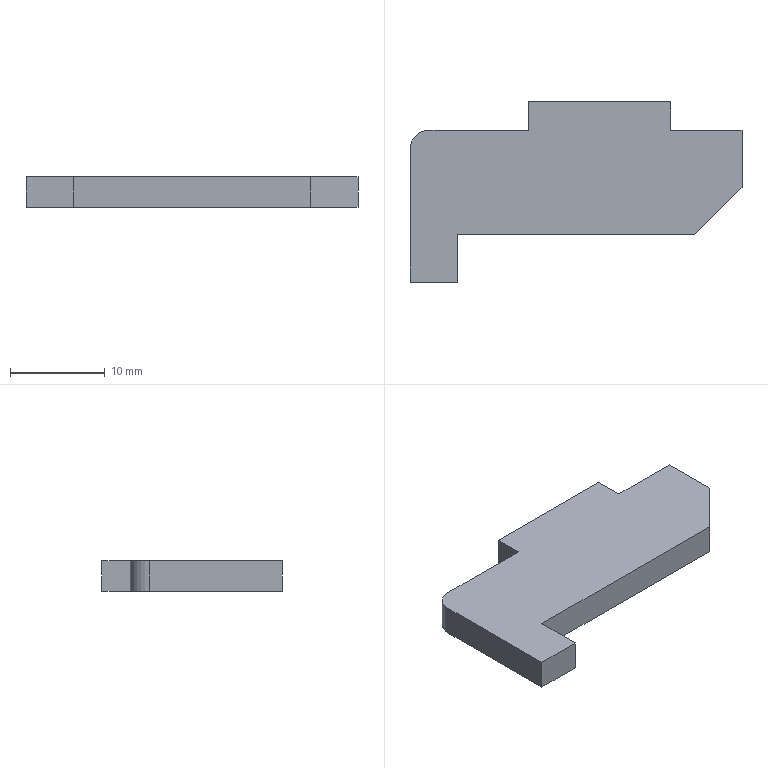Part | SolidWorks | features FlatPattern 1, SMBaseFlange 1, SheetMetal 1 | 1 solid | 14 faces | box 35 x 19 x 3.2 mm | volume 1413 mm3 | plane 13 | cylinder 1 | commonest cylinder face diameters 4 x1
STEP:
#1=CARTESIAN_POINT('',(-81.748,-105.118,0.));
#2=VERTEX_POINT('',#1);
#3=CARTESIAN_POINT('',(-81.748,-100.118,0.));
#4=VERTEX_POINT('',#3);
#5=CARTESIAN_POINT('',(-81.748,-100.118,0.));
#6=DIRECTION('',(0.,1.,0.));
#7=VECTOR('',#6,1000.);
#8=LINE('',#5,#7);
#9=EDGE_CURVE('',#2,#4,#8,.T.);
#10=ORIENTED_EDGE('',*,*,#9,.F.);
#11=CARTESIAN_POINT('',(-81.748,-105.118,-3.2));
#12=VERTEX_POINT('',#11);
#13=CARTESIAN_POINT('',(-81.748,-105.118,-3.2));
#14=DIRECTION('',(0.,0.,1.));
#15=VECTOR('',#14,1000.);
#16=LINE('',#13,#15);
#17=EDGE_CURVE('',#12,#2,#16,.T.);
#18=ORIENTED_EDGE('',*,*,#17,.F.);
#19=CARTESIAN_POINT('',(-81.748,-100.118,-3.2));
#20=VERTEX_POINT('',#19);
#21=CARTESIAN_POINT('',(-81.748,-100.118,-3.2));
#22=DIRECTION('',(0.,1.,0.));
#23=VECTOR('',#22,1000.);
#24=LINE('',#21,#23);
#25=EDGE_CURVE('',#12,#20,#24,.T.);
#26=ORIENTED_EDGE('',*,*,#25,.T.);
#27=CARTESIAN_POINT('',(-81.748,-100.118,-3.2));
#28=DIRECTION('',(0.,0.,1.));
#29=VECTOR('',#28,1000.);
#30=LINE('',#27,#29);
#31=EDGE_CURVE('',#20,#4,#30,.T.);
#32=ORIENTED_EDGE('',*,*,#31,.T.);
#33=EDGE_LOOP('',(#10,#18,#26,#32));
#34=FACE_OUTER_BOUND('',#33,.T.);
#35=CARTESIAN_POINT('',(-81.748,-100.118,-3.2));
#36=DIRECTION('',(1.,0.,0.));
#37=DIRECTION('',(0.,0.,-1.));
#38=AXIS2_PLACEMENT_3D('',#35,#36,#37);
#39=PLANE('',#38);
#40=ADVANCED_FACE('',(#34),#39,.T.);
#41=CARTESIAN_POINT('',(-86.748,-105.118,0.));
#42=VERTEX_POINT('',#41);
#43=CARTESIAN_POINT('',(-81.748,-105.118,0.));
#44=DIRECTION('',(1.,0.,0.));
#45=VECTOR('',#44,1000.);
#46=LINE('',#43,#45);
#47=EDGE_CURVE('',#42,#2,#46,.T.);
#48=ORIENTED_EDGE('',*,*,#47,.F.);
#49=CARTESIAN_POINT('',(-86.748,-105.118,-3.2));
#50=VERTEX_POINT('',#49);
#51=CARTESIAN_POINT('',(-86.748,-105.118,-3.2));
#52=DIRECTION('',(0.,0.,1.));
#53=VECTOR('',#52,1000.);
#54=LINE('',#51,#53);
#55=EDGE_CURVE('',#50,#42,#54,.T.);
#56=ORIENTED_EDGE('',*,*,#55,.F.);
#57=CARTESIAN_POINT('',(-81.748,-105.118,-3.2));
#58=DIRECTION('',(1.,0.,0.));
#59=VECTOR('',#58,1000.);
#60=LINE('',#57,#59);
#61=EDGE_CURVE('',#50,#12,#60,.T.);
#62=ORIENTED_EDGE('',*,*,#61,.T.);
#63=ORIENTED_EDGE('',*,*,#17,.T.);
#64=EDGE_LOOP('',(#48,#56,#62,#63));
#65=FACE_OUTER_BOUND('',#64,.T.);
#66=CARTESIAN_POINT('',(-81.748,-105.118,-3.2));
#67=DIRECTION('',(0.,-1.,0.));
#68=DIRECTION('',(0.,0.,-1.));
#69=AXIS2_PLACEMENT_3D('',#66,#67,#68);
#70=PLANE('',#69);
#71=ADVANCED_FACE('',(#65),#70,.T.);
#72=CARTESIAN_POINT('',(-86.748,-91.118,0.));
#73=VERTEX_POINT('',#72);
#74=CARTESIAN_POINT('',(-86.748,-105.118,0.));
#75=DIRECTION('',(0.,-1.,0.));
#76=VECTOR('',#75,1000.);
#77=LINE('',#74,#76);
#78=EDGE_CURVE('',#73,#42,#77,.T.);
#79=ORIENTED_EDGE('',*,*,#78,.F.);
#80=CARTESIAN_POINT('',(-86.748,-91.118,-3.2));
#81=VERTEX_POINT('',#80);
#82=CARTESIAN_POINT('',(-86.748,-91.118,-3.2));
#83=DIRECTION('',(0.,0.,1.));
#84=VECTOR('',#83,1000.);
#85=LINE('',#82,#84);
#86=EDGE_CURVE('',#81,#73,#85,.T.);
#87=ORIENTED_EDGE('',*,*,#86,.F.);
#88=CARTESIAN_POINT('',(-86.748,-105.118,-3.2));
#89=DIRECTION('',(0.,-1.,0.));
#90=VECTOR('',#89,1000.);
#91=LINE('',#88,#90);
#92=EDGE_CURVE('',#81,#50,#91,.T.);
#93=ORIENTED_EDGE('',*,*,#92,.T.);
#94=ORIENTED_EDGE('',*,*,#55,.T.);
#95=EDGE_LOOP('',(#79,#87,#93,#94));
#96=FACE_OUTER_BOUND('',#95,.T.);
#97=CARTESIAN_POINT('',(-86.748,-105.118,-3.2));
#98=DIRECTION('',(-1.,0.,0.));
#99=DIRECTION('',(0.,0.,1.));
#100=AXIS2_PLACEMENT_3D('',#97,#98,#99);
#101=PLANE('',#100);
#102=ADVANCED_FACE('',(#96),#101,.T.);
#103=CARTESIAN_POINT('',(-84.748,-89.118,0.));
#104=VERTEX_POINT('',#103);
#105=CARTESIAN_POINT('',(-84.748,-91.118,0.));
#106=DIRECTION('',(0.,0.,1.));
#107=DIRECTION('',(-1.,0.,0.));
#108=AXIS2_PLACEMENT_3D('',#105,#106,#107);
#109=CIRCLE('',#108,2.);
#110=EDGE_CURVE('',#104,#73,#109,.T.);
#111=ORIENTED_EDGE('',*,*,#110,.F.);
#112=CARTESIAN_POINT('',(-84.748,-89.118,-3.2));
#113=VERTEX_POINT('',#112);
#114=CARTESIAN_POINT('',(-84.748,-89.118,-3.2));
#115=DIRECTION('',(0.,0.,1.));
#116=VECTOR('',#115,1000.);
#117=LINE('',#114,#116);
#118=EDGE_CURVE('',#113,#104,#117,.T.);
#119=ORIENTED_EDGE('',*,*,#118,.F.);
#120=CARTESIAN_POINT('',(-84.748,-91.118,-3.2));
#121=DIRECTION('',(0.,0.,1.));
#122=DIRECTION('',(-1.,0.,0.));
#123=AXIS2_PLACEMENT_3D('',#120,#121,#122);
#124=CIRCLE('',#123,2.);
#125=EDGE_CURVE('',#113,#81,#124,.T.);
#126=ORIENTED_EDGE('',*,*,#125,.T.);
#127=ORIENTED_EDGE('',*,*,#86,.T.);
#128=EDGE_LOOP('',(#111,#119,#126,#127));
#129=FACE_OUTER_BOUND('',#128,.T.);
#130=CARTESIAN_POINT('',(-84.748,-91.118,-3.2));
#131=DIRECTION('',(0.,0.,1.));
#132=DIRECTION('',(1.,0.,0.));
#133=AXIS2_PLACEMENT_3D('',#130,#131,#132);
#134=CYLINDRICAL_SURFACE('',#133,2.);
#135=ADVANCED_FACE('',(#129),#134,.T.);
#136=CARTESIAN_POINT('',(-74.248,-89.118,0.));
#137=VERTEX_POINT('',#136);
#138=CARTESIAN_POINT('',(-84.748,-89.118,0.));
#139=DIRECTION('',(-1.,0.,0.));
#140=VECTOR('',#139,1000.);
#141=LINE('',#138,#140);
#142=EDGE_CURVE('',#137,#104,#141,.T.);
#143=ORIENTED_EDGE('',*,*,#142,.F.);
#144=CARTESIAN_POINT('',(-74.248,-89.118,-3.2));
#145=VERTEX_POINT('',#144);
#146=CARTESIAN_POINT('',(-74.248,-89.118,-3.2));
#147=DIRECTION('',(0.,0.,1.));
#148=VECTOR('',#147,1000.);
#149=LINE('',#146,#148);
#150=EDGE_CURVE('',#145,#137,#149,.T.);
#151=ORIENTED_EDGE('',*,*,#150,.F.);
#152=CARTESIAN_POINT('',(-84.748,-89.118,-3.2));
#153=DIRECTION('',(-1.,0.,0.));
#154=VECTOR('',#153,1000.);
#155=LINE('',#152,#154);
#156=EDGE_CURVE('',#145,#113,#155,.T.);
#157=ORIENTED_EDGE('',*,*,#156,.T.);
#158=ORIENTED_EDGE('',*,*,#118,.T.);
#159=EDGE_LOOP('',(#143,#151,#157,#158));
#160=FACE_OUTER_BOUND('',#159,.T.);
#161=CARTESIAN_POINT('',(-84.748,-89.118,-3.2));
#162=DIRECTION('',(0.,1.,0.));
#163=DIRECTION('',(0.,0.,1.));
#164=AXIS2_PLACEMENT_3D('',#161,#162,#163);
#165=PLANE('',#164);
#166=ADVANCED_FACE('',(#160),#165,.T.);
#167=CARTESIAN_POINT('',(-74.248,-86.118,0.));
#168=VERTEX_POINT('',#167);
#169=CARTESIAN_POINT('',(-74.248,-89.118,0.));
#170=DIRECTION('',(0.,-1.,0.));
#171=VECTOR('',#170,1000.);
#172=LINE('',#169,#171);
#173=EDGE_CURVE('',#168,#137,#172,.T.);
#174=ORIENTED_EDGE('',*,*,#173,.F.);
#175=CARTESIAN_POINT('',(-74.248,-86.118,-3.2));
#176=VERTEX_POINT('',#175);
#177=CARTESIAN_POINT('',(-74.248,-86.118,-3.2));
#178=DIRECTION('',(0.,0.,1.));
#179=VECTOR('',#178,1000.);
#180=LINE('',#177,#179);
#181=EDGE_CURVE('',#176,#168,#180,.T.);
#182=ORIENTED_EDGE('',*,*,#181,.F.);
#183=CARTESIAN_POINT('',(-74.248,-89.118,-3.2));
#184=DIRECTION('',(0.,-1.,0.));
#185=VECTOR('',#184,1000.);
#186=LINE('',#183,#185);
#187=EDGE_CURVE('',#176,#145,#186,.T.);
#188=ORIENTED_EDGE('',*,*,#187,.T.);
#189=ORIENTED_EDGE('',*,*,#150,.T.);
#190=EDGE_LOOP('',(#174,#182,#188,#189));
#191=FACE_OUTER_BOUND('',#190,.T.);
#192=CARTESIAN_POINT('',(-74.248,-89.118,-3.2));
#193=DIRECTION('',(-1.,0.,0.));
#194=DIRECTION('',(0.,0.,1.));
#195=AXIS2_PLACEMENT_3D('',#192,#193,#194);
#196=PLANE('',#195);
#197=ADVANCED_FACE('',(#191),#196,.T.);
#198=CARTESIAN_POINT('',(-59.248,-86.118,0.));
#199=VERTEX_POINT('',#198);
#200=CARTESIAN_POINT('',(-74.248,-86.118,0.));
#201=DIRECTION('',(-1.,0.,0.));
#202=VECTOR('',#201,1000.);
#203=LINE('',#200,#202);
#204=EDGE_CURVE('',#199,#168,#203,.T.);
#205=ORIENTED_EDGE('',*,*,#204,.F.);
#206=CARTESIAN_POINT('',(-59.248,-86.118,-3.2));
#207=VERTEX_POINT('',#206);
#208=CARTESIAN_POINT('',(-59.248,-86.118,-3.2));
#209=DIRECTION('',(0.,0.,1.));
#210=VECTOR('',#209,1000.);
#211=LINE('',#208,#210);
#212=EDGE_CURVE('',#207,#199,#211,.T.);
#213=ORIENTED_EDGE('',*,*,#212,.F.);
#214=CARTESIAN_POINT('',(-74.248,-86.118,-3.2));
#215=DIRECTION('',(-1.,0.,0.));
#216=VECTOR('',#215,1000.);
#217=LINE('',#214,#216);
#218=EDGE_CURVE('',#207,#176,#217,.T.);
#219=ORIENTED_EDGE('',*,*,#218,.T.);
#220=ORIENTED_EDGE('',*,*,#181,.T.);
#221=EDGE_LOOP('',(#205,#213,#219,#220));
#222=FACE_OUTER_BOUND('',#221,.T.);
#223=CARTESIAN_POINT('',(-74.248,-86.118,-3.2));
#224=DIRECTION('',(0.,1.,0.));
#225=DIRECTION('',(0.,0.,1.));
#226=AXIS2_PLACEMENT_3D('',#223,#224,#225);
#227=PLANE('',#226);
#228=ADVANCED_FACE('',(#222),#227,.T.);
#229=CARTESIAN_POINT('',(-59.248,-89.118,0.));
#230=VERTEX_POINT('',#229);
#231=CARTESIAN_POINT('',(-59.248,-86.118,0.));
#232=DIRECTION('',(0.,1.,0.));
#233=VECTOR('',#232,1000.);
#234=LINE('',#231,#233);
#235=EDGE_CURVE('',#230,#199,#234,.T.);
#236=ORIENTED_EDGE('',*,*,#235,.F.);
#237=CARTESIAN_POINT('',(-59.248,-89.118,-3.2));
#238=VERTEX_POINT('',#237);
#239=CARTESIAN_POINT('',(-59.248,-89.118,-3.2));
#240=DIRECTION('',(0.,0.,1.));
#241=VECTOR('',#240,1000.);
#242=LINE('',#239,#241);
#243=EDGE_CURVE('',#238,#230,#242,.T.);
#244=ORIENTED_EDGE('',*,*,#243,.F.);
#245=CARTESIAN_POINT('',(-59.248,-86.118,-3.2));
#246=DIRECTION('',(0.,1.,0.));
#247=VECTOR('',#246,1000.);
#248=LINE('',#245,#247);
#249=EDGE_CURVE('',#238,#207,#248,.T.);
#250=ORIENTED_EDGE('',*,*,#249,.T.);
#251=ORIENTED_EDGE('',*,*,#212,.T.);
#252=EDGE_LOOP('',(#236,#244,#250,#251));
#253=FACE_OUTER_BOUND('',#252,.T.);
#254=CARTESIAN_POINT('',(-59.248,-86.118,-3.2));
#255=DIRECTION('',(1.,0.,0.));
#256=DIRECTION('',(0.,0.,-1.));
#257=AXIS2_PLACEMENT_3D('',#254,#255,#256);
#258=PLANE('',#257);
#259=ADVANCED_FACE('',(#253),#258,.T.);
#260=CARTESIAN_POINT('',(-51.748,-89.118,0.));
#261=VERTEX_POINT('',#260);
#262=CARTESIAN_POINT('',(-59.248,-89.118,0.));
#263=DIRECTION('',(-1.,0.,0.));
#264=VECTOR('',#263,1000.);
#265=LINE('',#262,#264);
#266=EDGE_CURVE('',#261,#230,#265,.T.);
#267=ORIENTED_EDGE('',*,*,#266,.F.);
#268=CARTESIAN_POINT('',(-51.748,-89.118,-3.2));
#269=VERTEX_POINT('',#268);
#270=CARTESIAN_POINT('',(-51.748,-89.118,-3.2));
#271=DIRECTION('',(0.,0.,1.));
#272=VECTOR('',#271,1000.);
#273=LINE('',#270,#272);
#274=EDGE_CURVE('',#269,#261,#273,.T.);
#275=ORIENTED_EDGE('',*,*,#274,.F.);
#276=CARTESIAN_POINT('',(-59.248,-89.118,-3.2));
#277=DIRECTION('',(-1.,0.,0.));
#278=VECTOR('',#277,1000.);
#279=LINE('',#276,#278);
#280=EDGE_CURVE('',#269,#238,#279,.T.);
#281=ORIENTED_EDGE('',*,*,#280,.T.);
#282=ORIENTED_EDGE('',*,*,#243,.T.);
#283=EDGE_LOOP('',(#267,#275,#281,#282));
#284=FACE_OUTER_BOUND('',#283,.T.);
#285=CARTESIAN_POINT('',(-59.248,-89.118,-3.2));
#286=DIRECTION('',(0.,1.,0.));
#287=DIRECTION('',(0.,0.,1.));
#288=AXIS2_PLACEMENT_3D('',#285,#286,#287);
#289=PLANE('',#288);
#290=ADVANCED_FACE('',(#284),#289,.T.);
#291=CARTESIAN_POINT('',(-51.748,-95.118,0.));
#292=VERTEX_POINT('',#291);
#293=CARTESIAN_POINT('',(-51.748,-89.118,0.));
#294=DIRECTION('',(0.,1.,0.));
#295=VECTOR('',#294,1000.);
#296=LINE('',#293,#295);
#297=EDGE_CURVE('',#292,#261,#296,.T.);
#298=ORIENTED_EDGE('',*,*,#297,.F.);
#299=CARTESIAN_POINT('',(-51.748,-95.118,-3.2));
#300=VERTEX_POINT('',#299);
#301=CARTESIAN_POINT('',(-51.748,-95.118,-3.2));
#302=DIRECTION('',(0.,0.,1.));
#303=VECTOR('',#302,1000.);
#304=LINE('',#301,#303);
#305=EDGE_CURVE('',#300,#292,#304,.T.);
#306=ORIENTED_EDGE('',*,*,#305,.F.);
#307=CARTESIAN_POINT('',(-51.748,-89.118,-3.2));
#308=DIRECTION('',(0.,1.,0.));
#309=VECTOR('',#308,1000.);
#310=LINE('',#307,#309);
#311=EDGE_CURVE('',#300,#269,#310,.T.);
#312=ORIENTED_EDGE('',*,*,#311,.T.);
#313=ORIENTED_EDGE('',*,*,#274,.T.);
#314=EDGE_LOOP('',(#298,#306,#312,#313));
#315=FACE_OUTER_BOUND('',#314,.T.);
#316=CARTESIAN_POINT('',(-51.748,-89.118,-3.2));
#317=DIRECTION('',(1.,0.,0.));
#318=DIRECTION('',(0.,0.,-1.));
#319=AXIS2_PLACEMENT_3D('',#316,#317,#318);
#320=PLANE('',#319);
#321=ADVANCED_FACE('',(#315),#320,.T.);
#322=CARTESIAN_POINT('',(-56.748,-100.118,0.));
#323=VERTEX_POINT('',#322);
#324=CARTESIAN_POINT('',(-51.748,-95.118,0.));
#325=DIRECTION('',(0.7071,0.7071,0.));
#326=VECTOR('',#325,1000.);
#327=LINE('',#324,#326);
#328=EDGE_CURVE('',#323,#292,#327,.T.);
#329=ORIENTED_EDGE('',*,*,#328,.F.);
#330=CARTESIAN_POINT('',(-56.748,-100.118,-3.2));
#331=VERTEX_POINT('',#330);
#332=CARTESIAN_POINT('',(-56.748,-100.118,-3.2));
#333=DIRECTION('',(0.,0.,1.));
#334=VECTOR('',#333,1000.);
#335=LINE('',#332,#334);
#336=EDGE_CURVE('',#331,#323,#335,.T.);
#337=ORIENTED_EDGE('',*,*,#336,.F.);
#338=CARTESIAN_POINT('',(-51.748,-95.118,-3.2));
#339=DIRECTION('',(0.7071,0.7071,0.));
#340=VECTOR('',#339,1000.);
#341=LINE('',#338,#340);
#342=EDGE_CURVE('',#331,#300,#341,.T.);
#343=ORIENTED_EDGE('',*,*,#342,.T.);
#344=ORIENTED_EDGE('',*,*,#305,.T.);
#345=EDGE_LOOP('',(#329,#337,#343,#344));
#346=FACE_OUTER_BOUND('',#345,.T.);
#347=CARTESIAN_POINT('',(-51.748,-95.118,-3.2));
#348=DIRECTION('',(0.7071,-0.7071,0.));
#349=DIRECTION('',(0.7071,0.7071,0.));
#350=AXIS2_PLACEMENT_3D('',#347,#348,#349);
#351=PLANE('',#350);
#352=ADVANCED_FACE('',(#346),#351,.T.);
#353=CARTESIAN_POINT('',(-56.748,-100.118,0.));
#354=DIRECTION('',(1.,0.,0.));
#355=VECTOR('',#354,1000.);
#356=LINE('',#353,#355);
#357=EDGE_CURVE('',#4,#323,#356,.T.);
#358=ORIENTED_EDGE('',*,*,#357,.F.);
#359=ORIENTED_EDGE('',*,*,#31,.F.);
#360=CARTESIAN_POINT('',(-56.748,-100.118,-3.2));
#361=DIRECTION('',(1.,0.,0.));
#362=VECTOR('',#361,1000.);
#363=LINE('',#360,#362);
#364=EDGE_CURVE('',#20,#331,#363,.T.);
#365=ORIENTED_EDGE('',*,*,#364,.T.);
#366=ORIENTED_EDGE('',*,*,#336,.T.);
#367=EDGE_LOOP('',(#358,#359,#365,#366));
#368=FACE_OUTER_BOUND('',#367,.T.);
#369=CARTESIAN_POINT('',(-56.748,-100.118,-3.2));
#370=DIRECTION('',(0.,-1.,0.));
#371=DIRECTION('',(0.,0.,-1.));
#372=AXIS2_PLACEMENT_3D('',#369,#370,#371);
#373=PLANE('',#372);
#374=ADVANCED_FACE('',(#368),#373,.T.);
#375=ORIENTED_EDGE('',*,*,#25,.F.);
#376=ORIENTED_EDGE('',*,*,#61,.F.);
#377=ORIENTED_EDGE('',*,*,#92,.F.);
#378=ORIENTED_EDGE('',*,*,#125,.F.);
#379=ORIENTED_EDGE('',*,*,#156,.F.);
#380=ORIENTED_EDGE('',*,*,#187,.F.);
#381=ORIENTED_EDGE('',*,*,#218,.F.);
#382=ORIENTED_EDGE('',*,*,#249,.F.);
#383=ORIENTED_EDGE('',*,*,#280,.F.);
#384=ORIENTED_EDGE('',*,*,#311,.F.);
#385=ORIENTED_EDGE('',*,*,#342,.F.);
#386=ORIENTED_EDGE('',*,*,#364,.F.);
#387=EDGE_LOOP('',(#375,#376,#377,#378,#379,#380,#381,#382,#383,#384,#385,#386));
#388=FACE_OUTER_BOUND('',#387,.T.);
#389=CARTESIAN_POINT('',(-84.748,-91.118,-3.2));
#390=DIRECTION('',(0.,0.,-1.));
#391=DIRECTION('',(-1.,0.,0.));
#392=AXIS2_PLACEMENT_3D('',#389,#390,#391);
#393=PLANE('',#392);
#394=ADVANCED_FACE('',(#388),#393,.T.);
#395=ORIENTED_EDGE('',*,*,#9,.T.);
#396=ORIENTED_EDGE('',*,*,#357,.T.);
#397=ORIENTED_EDGE('',*,*,#328,.T.);
#398=ORIENTED_EDGE('',*,*,#297,.T.);
#399=ORIENTED_EDGE('',*,*,#266,.T.);
#400=ORIENTED_EDGE('',*,*,#235,.T.);
#401=ORIENTED_EDGE('',*,*,#204,.T.);
#402=ORIENTED_EDGE('',*,*,#173,.T.);
#403=ORIENTED_EDGE('',*,*,#142,.T.);
#404=ORIENTED_EDGE('',*,*,#110,.T.);
#405=ORIENTED_EDGE('',*,*,#78,.T.);
#406=ORIENTED_EDGE('',*,*,#47,.T.);
#407=EDGE_LOOP('',(#395,#396,#397,#398,#399,#400,#401,#402,#403,#404,#405,#406));
#408=FACE_OUTER_BOUND('',#407,.T.);
#409=CARTESIAN_POINT('',(-84.748,-91.118,0.));
#410=DIRECTION('',(0.,0.,-1.));
#411=DIRECTION('',(-1.,0.,0.));
#412=AXIS2_PLACEMENT_3D('',#409,#410,#411);
#413=PLANE('',#412);
#414=ADVANCED_FACE('',(#408),#413,.F.);
#415=CLOSED_SHELL('',(#40,#71,#102,#135,#166,#197,#228,#259,#290,#321,#352,#374,#394,#414));
#416=MANIFOLD_SOLID_BREP('',#415);
#417=CARTESIAN_POINT('',(0.,0.,0.));
#418=DIRECTION('',(0.,0.,1.));
#419=DIRECTION('',(1.,0.,0.));
#420=AXIS2_PLACEMENT_3D('',#417,#418,#419);
#421=(LENGTH_UNIT()NAMED_UNIT(*)SI_UNIT(.MILLI.,.METRE.));
#422=UNCERTAINTY_MEASURE_WITH_UNIT(LENGTH_MEASURE(0.00001),#421,'','');
#423=(NAMED_UNIT(*)PLANE_ANGLE_UNIT()SI_UNIT($,.RADIAN.));
#424=(NAMED_UNIT(*)SI_UNIT($,.STERADIAN.)SOLID_ANGLE_UNIT());
#425=(GEOMETRIC_REPRESENTATION_CONTEXT(3)GLOBAL_UNCERTAINTY_ASSIGNED_CONTEXT((#422))GLOBAL_UNIT_ASSIGNED_CONTEXT((#421,#423,#424))REPRESENTATION_CONTEXT('',''));
#426=ADVANCED_BREP_SHAPE_REPRESENTATION('',(#416,#420),#425);